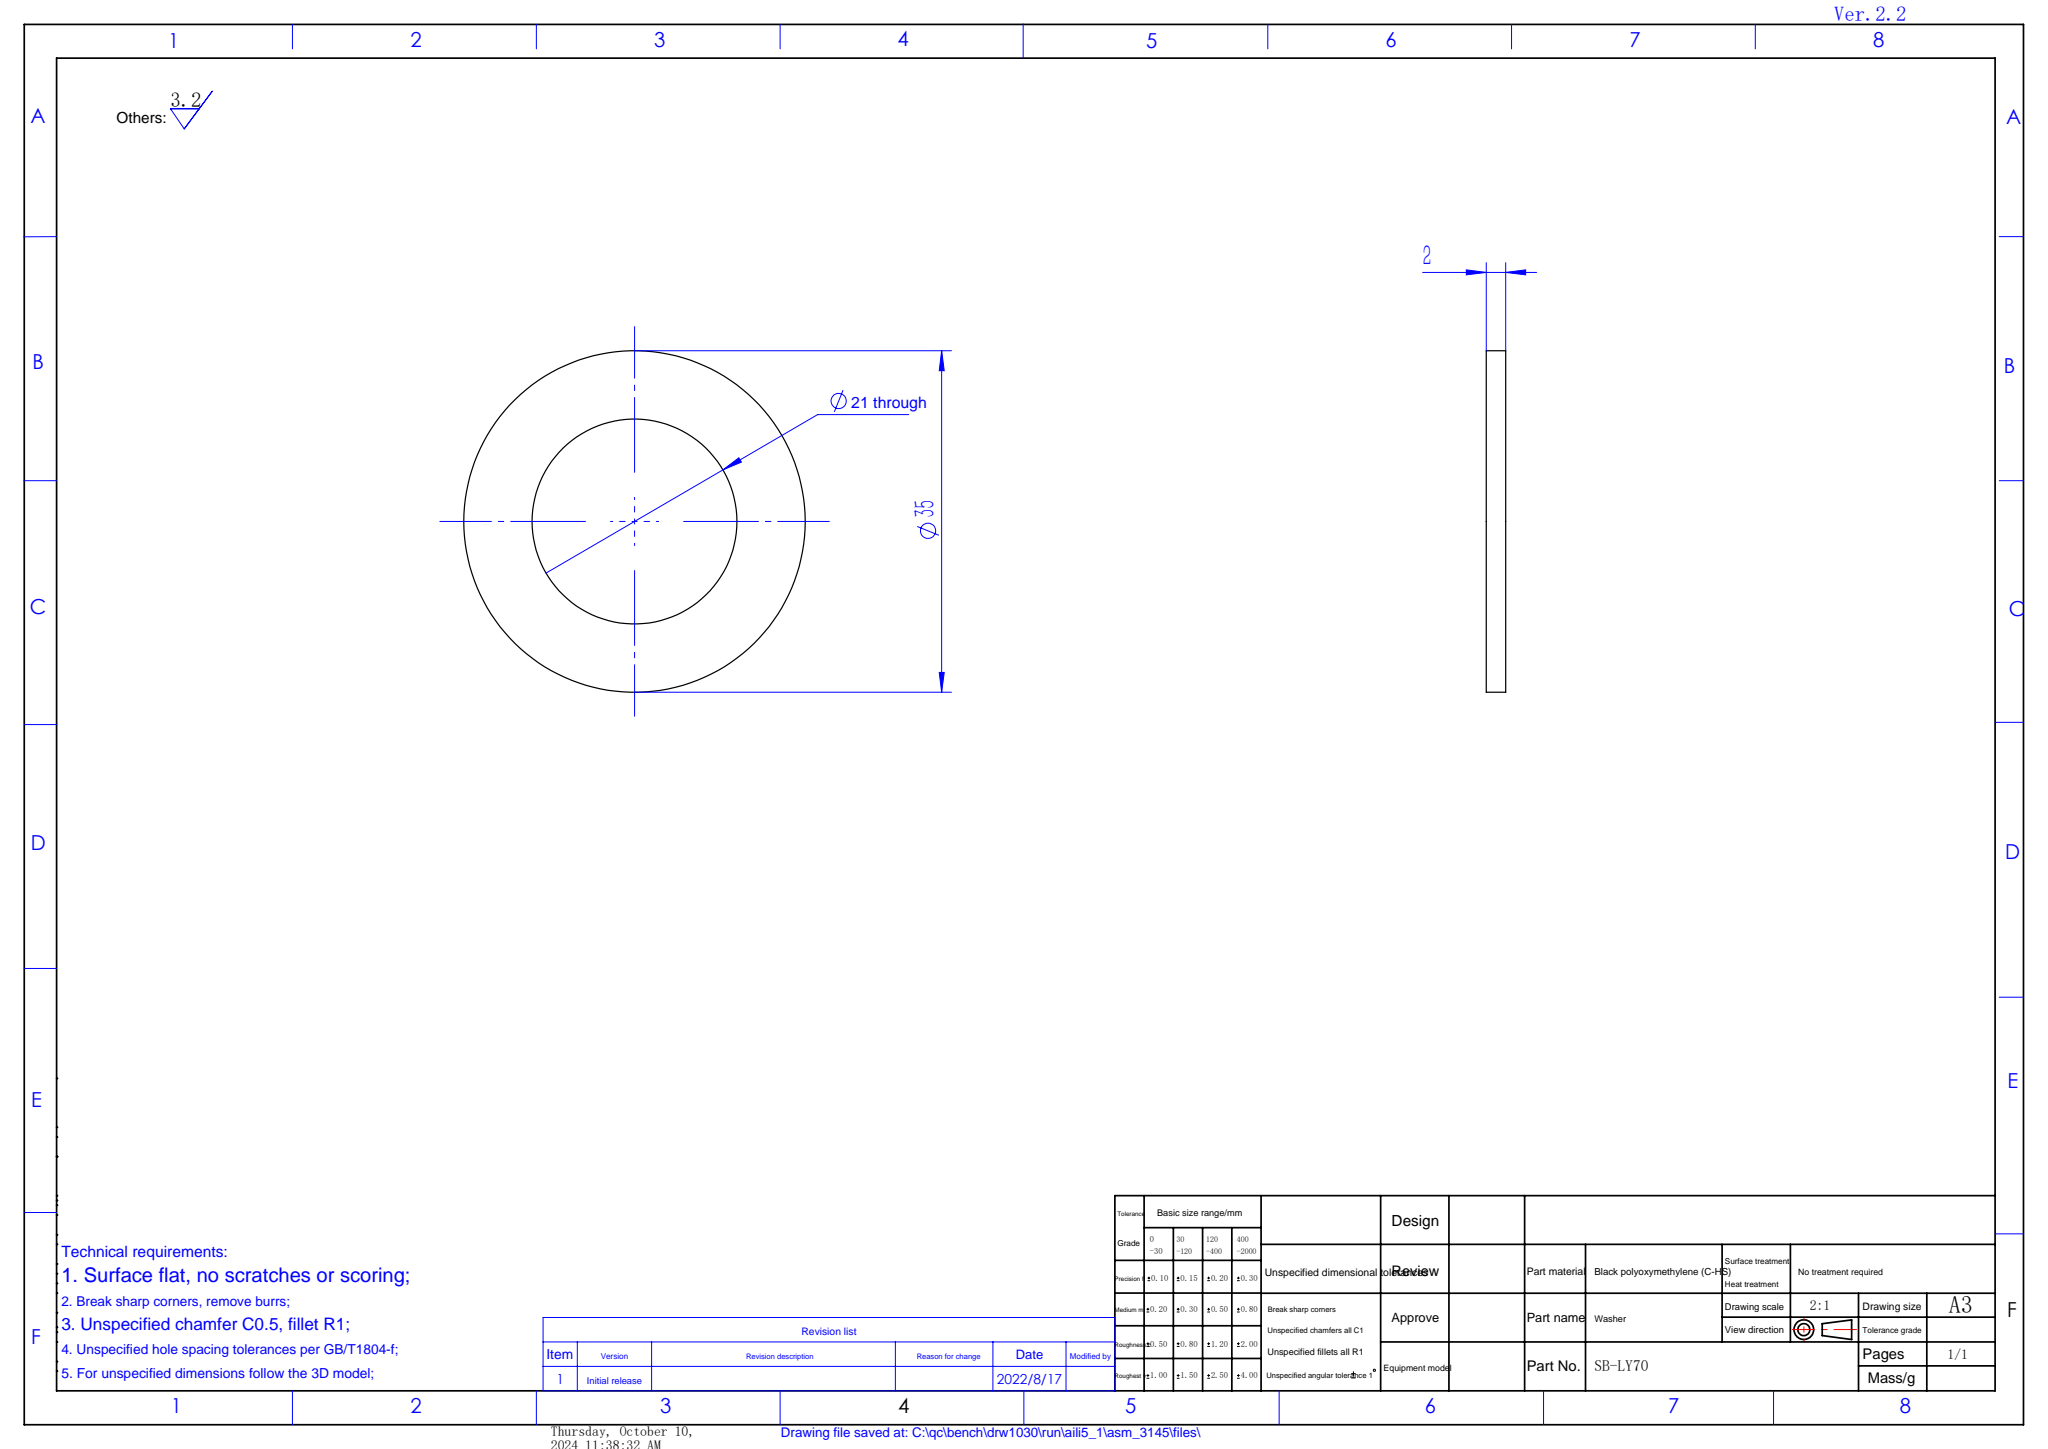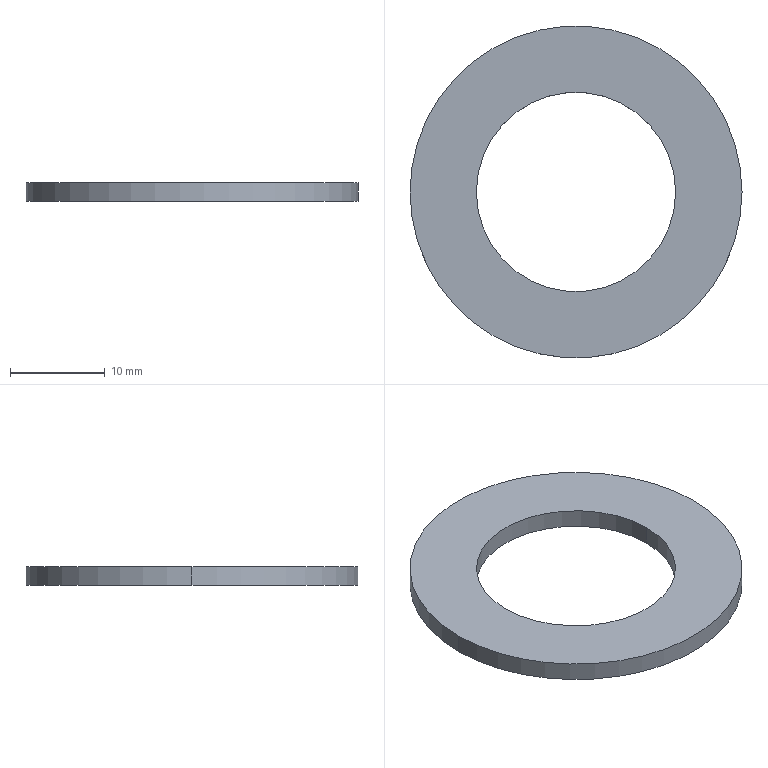Part | SolidWorks | features Extrusion 1 | 1 solid | 6 faces | box 35 x 35 x 2 mm | volume 1232 mm3 | cylinder 4 | plane 2 | commonest cylinder face diameters 21 x2 35 x2
STEP:
#1=CARTESIAN_POINT('',(-10.5,0.,2.));
#2=VERTEX_POINT('',#1);
#3=CARTESIAN_POINT('',(10.5,0.,2.));
#4=VERTEX_POINT('',#3);
#5=CARTESIAN_POINT('',(0.,0.,2.));
#6=DIRECTION('',(0.,0.,1.));
#7=DIRECTION('',(1.,0.,0.));
#8=AXIS2_PLACEMENT_3D('',#5,#6,#7);
#9=CIRCLE('',#8,10.5);
#10=EDGE_CURVE('',#2,#4,#9,.T.);
#11=ORIENTED_EDGE('',*,*,#10,.T.);
#12=CARTESIAN_POINT('',(10.5,0.,0.));
#13=VERTEX_POINT('',#12);
#14=CARTESIAN_POINT('',(10.5,0.,2.));
#15=DIRECTION('',(0.,0.,-1.));
#16=VECTOR('',#15,1000.);
#17=LINE('',#14,#16);
#18=EDGE_CURVE('',#4,#13,#17,.T.);
#19=ORIENTED_EDGE('',*,*,#18,.T.);
#20=CARTESIAN_POINT('',(-10.5,0.,0.));
#21=VERTEX_POINT('',#20);
#22=CARTESIAN_POINT('',(0.,0.,0.));
#23=DIRECTION('',(0.,0.,1.));
#24=DIRECTION('',(1.,0.,0.));
#25=AXIS2_PLACEMENT_3D('',#22,#23,#24);
#26=CIRCLE('',#25,10.5);
#27=EDGE_CURVE('',#21,#13,#26,.T.);
#28=ORIENTED_EDGE('',*,*,#27,.F.);
#29=CARTESIAN_POINT('',(-10.5,0.,2.));
#30=DIRECTION('',(0.,0.,-1.));
#31=VECTOR('',#30,1000.);
#32=LINE('',#29,#31);
#33=EDGE_CURVE('',#2,#21,#32,.T.);
#34=ORIENTED_EDGE('',*,*,#33,.F.);
#35=EDGE_LOOP('',(#11,#19,#28,#34));
#36=FACE_OUTER_BOUND('',#35,.T.);
#37=CARTESIAN_POINT('',(0.,0.,2.));
#38=DIRECTION('',(0.,0.,-1.));
#39=DIRECTION('',(-1.,0.,0.));
#40=AXIS2_PLACEMENT_3D('',#37,#38,#39);
#41=CYLINDRICAL_SURFACE('',#40,10.5);
#42=ADVANCED_FACE('',(#36),#41,.F.);
#43=CARTESIAN_POINT('',(17.5,0.,2.));
#44=VERTEX_POINT('',#43);
#45=CARTESIAN_POINT('',(-17.5,0.,2.));
#46=VERTEX_POINT('',#45);
#47=CARTESIAN_POINT('',(0.,0.,2.));
#48=DIRECTION('',(0.,0.,1.));
#49=DIRECTION('',(1.,0.,0.));
#50=AXIS2_PLACEMENT_3D('',#47,#48,#49);
#51=CIRCLE('',#50,17.5);
#52=EDGE_CURVE('',#44,#46,#51,.T.);
#53=ORIENTED_EDGE('',*,*,#52,.F.);
#54=CARTESIAN_POINT('',(17.5,0.,0.));
#55=VERTEX_POINT('',#54);
#56=CARTESIAN_POINT('',(17.5,0.,2.));
#57=DIRECTION('',(0.,0.,-1.));
#58=VECTOR('',#57,1000.);
#59=LINE('',#56,#58);
#60=EDGE_CURVE('',#44,#55,#59,.T.);
#61=ORIENTED_EDGE('',*,*,#60,.T.);
#62=CARTESIAN_POINT('',(-17.5,0.,0.));
#63=VERTEX_POINT('',#62);
#64=CARTESIAN_POINT('',(0.,0.,0.));
#65=DIRECTION('',(0.,0.,1.));
#66=DIRECTION('',(1.,0.,0.));
#67=AXIS2_PLACEMENT_3D('',#64,#65,#66);
#68=CIRCLE('',#67,17.5);
#69=EDGE_CURVE('',#55,#63,#68,.T.);
#70=ORIENTED_EDGE('',*,*,#69,.T.);
#71=CARTESIAN_POINT('',(-17.5,0.,2.));
#72=DIRECTION('',(0.,0.,-1.));
#73=VECTOR('',#72,1000.);
#74=LINE('',#71,#73);
#75=EDGE_CURVE('',#46,#63,#74,.T.);
#76=ORIENTED_EDGE('',*,*,#75,.F.);
#77=EDGE_LOOP('',(#53,#61,#70,#76));
#78=FACE_OUTER_BOUND('',#77,.T.);
#79=CARTESIAN_POINT('',(0.,0.,2.));
#80=DIRECTION('',(0.,0.,-1.));
#81=DIRECTION('',(-1.,0.,0.));
#82=AXIS2_PLACEMENT_3D('',#79,#80,#81);
#83=CYLINDRICAL_SURFACE('',#82,17.5);
#84=ADVANCED_FACE('',(#78),#83,.T.);
#85=CARTESIAN_POINT('',(0.,0.,2.));
#86=DIRECTION('',(0.,0.,1.));
#87=DIRECTION('',(1.,0.,0.));
#88=AXIS2_PLACEMENT_3D('',#85,#86,#87);
#89=CIRCLE('',#88,17.5);
#90=EDGE_CURVE('',#46,#44,#89,.T.);
#91=ORIENTED_EDGE('',*,*,#90,.T.);
#92=ORIENTED_EDGE('',*,*,#52,.T.);
#93=EDGE_LOOP('',(#91,#92));
#94=FACE_OUTER_BOUND('',#93,.T.);
#95=ORIENTED_EDGE('',*,*,#10,.F.);
#96=CARTESIAN_POINT('',(0.,0.,2.));
#97=DIRECTION('',(0.,0.,1.));
#98=DIRECTION('',(1.,0.,0.));
#99=AXIS2_PLACEMENT_3D('',#96,#97,#98);
#100=CIRCLE('',#99,10.5);
#101=EDGE_CURVE('',#4,#2,#100,.T.);
#102=ORIENTED_EDGE('',*,*,#101,.F.);
#103=EDGE_LOOP('',(#95,#102));
#104=FACE_BOUND('',#103,.T.);
#105=CARTESIAN_POINT('',(0.,0.,2.));
#106=DIRECTION('',(0.,0.,1.));
#107=DIRECTION('',(1.,0.,0.));
#108=AXIS2_PLACEMENT_3D('',#105,#106,#107);
#109=PLANE('',#108);
#110=ADVANCED_FACE('',(#94,#104),#109,.T.);
#111=CARTESIAN_POINT('',(0.,0.,0.));
#112=DIRECTION('',(0.,0.,1.));
#113=DIRECTION('',(1.,0.,0.));
#114=AXIS2_PLACEMENT_3D('',#111,#112,#113);
#115=CIRCLE('',#114,17.5);
#116=EDGE_CURVE('',#63,#55,#115,.T.);
#117=ORIENTED_EDGE('',*,*,#116,.F.);
#118=ORIENTED_EDGE('',*,*,#69,.F.);
#119=EDGE_LOOP('',(#117,#118));
#120=FACE_OUTER_BOUND('',#119,.T.);
#121=ORIENTED_EDGE('',*,*,#27,.T.);
#122=CARTESIAN_POINT('',(0.,0.,0.));
#123=DIRECTION('',(0.,0.,1.));
#124=DIRECTION('',(1.,0.,0.));
#125=AXIS2_PLACEMENT_3D('',#122,#123,#124);
#126=CIRCLE('',#125,10.5);
#127=EDGE_CURVE('',#13,#21,#126,.T.);
#128=ORIENTED_EDGE('',*,*,#127,.T.);
#129=EDGE_LOOP('',(#121,#128));
#130=FACE_BOUND('',#129,.T.);
#131=CARTESIAN_POINT('',(0.,0.,0.));
#132=DIRECTION('',(0.,0.,1.));
#133=DIRECTION('',(1.,0.,0.));
#134=AXIS2_PLACEMENT_3D('',#131,#132,#133);
#135=PLANE('',#134);
#136=ADVANCED_FACE('',(#120,#130),#135,.F.);
#137=ORIENTED_EDGE('',*,*,#60,.F.);
#138=ORIENTED_EDGE('',*,*,#90,.F.);
#139=ORIENTED_EDGE('',*,*,#75,.T.);
#140=ORIENTED_EDGE('',*,*,#116,.T.);
#141=EDGE_LOOP('',(#137,#138,#139,#140));
#142=FACE_OUTER_BOUND('',#141,.T.);
#143=CARTESIAN_POINT('',(0.,0.,2.));
#144=DIRECTION('',(0.,0.,-1.));
#145=DIRECTION('',(-1.,0.,0.));
#146=AXIS2_PLACEMENT_3D('',#143,#144,#145);
#147=CYLINDRICAL_SURFACE('',#146,17.5);
#148=ADVANCED_FACE('',(#142),#147,.T.);
#149=ORIENTED_EDGE('',*,*,#18,.F.);
#150=ORIENTED_EDGE('',*,*,#101,.T.);
#151=ORIENTED_EDGE('',*,*,#33,.T.);
#152=ORIENTED_EDGE('',*,*,#127,.F.);
#153=EDGE_LOOP('',(#149,#150,#151,#152));
#154=FACE_OUTER_BOUND('',#153,.T.);
#155=CARTESIAN_POINT('',(0.,0.,2.));
#156=DIRECTION('',(0.,0.,-1.));
#157=DIRECTION('',(-1.,0.,0.));
#158=AXIS2_PLACEMENT_3D('',#155,#156,#157);
#159=CYLINDRICAL_SURFACE('',#158,10.5);
#160=ADVANCED_FACE('',(#154),#159,.F.);
#161=CLOSED_SHELL('',(#42,#84,#110,#136,#148,#160));
#162=MANIFOLD_SOLID_BREP('',#161);
#163=CARTESIAN_POINT('',(0.,0.,0.));
#164=DIRECTION('',(0.,0.,1.));
#165=DIRECTION('',(1.,0.,0.));
#166=AXIS2_PLACEMENT_3D('',#163,#164,#165);
#167=(LENGTH_UNIT()NAMED_UNIT(*)SI_UNIT(.MILLI.,.METRE.));
#168=UNCERTAINTY_MEASURE_WITH_UNIT(LENGTH_MEASURE(0.00001),#167,'','');
#169=(NAMED_UNIT(*)PLANE_ANGLE_UNIT()SI_UNIT($,.RADIAN.));
#170=(NAMED_UNIT(*)SI_UNIT($,.STERADIAN.)SOLID_ANGLE_UNIT());
#171=(GEOMETRIC_REPRESENTATION_CONTEXT(3)GLOBAL_UNCERTAINTY_ASSIGNED_CONTEXT((#168))GLOBAL_UNIT_ASSIGNED_CONTEXT((#167,#169,#170))REPRESENTATION_CONTEXT('',''));
#172=ADVANCED_BREP_SHAPE_REPRESENTATION('',(#162,#166),#171);